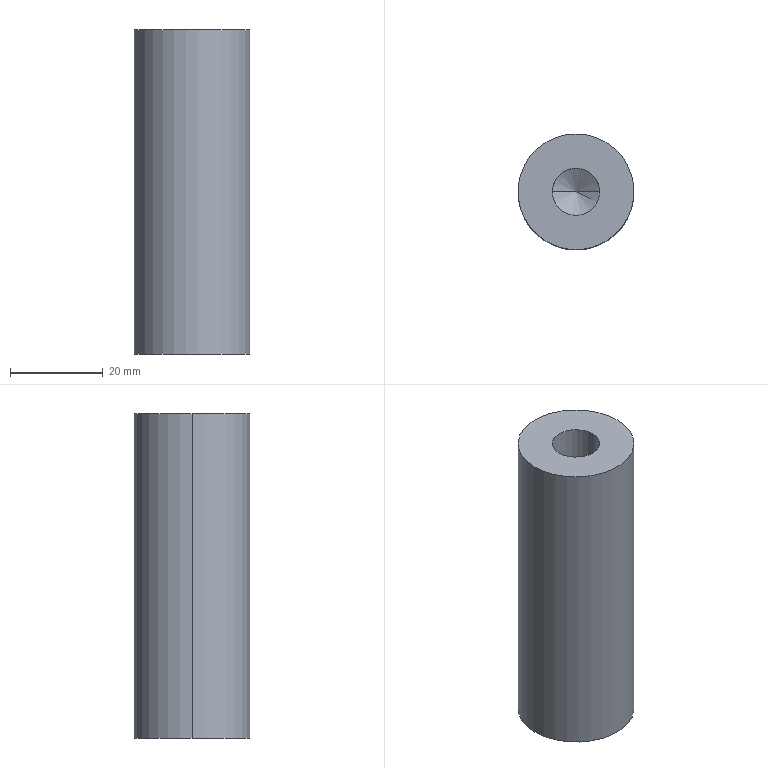Part | SolidWorks | features HoleWzd 2, Extrusion 1 | 1 solid | 12 faces | box 25 x 25 x 70 mm | volume 29291 mm3 | cylinder 6 | cone 4 | plane 2 | commonest cylinder face diameters 10.2 x4 25 x2
STEP:
#1=CARTESIAN_POINT('',(5.1,0.,30.));
#2=VERTEX_POINT('',#1);
#3=CARTESIAN_POINT('',(-5.1,0.,30.));
#4=VERTEX_POINT('',#3);
#5=CARTESIAN_POINT('',(0.,0.,30.));
#6=DIRECTION('',(0.,0.,-1.));
#7=DIRECTION('',(-1.,0.,0.));
#8=AXIS2_PLACEMENT_3D('',#5,#6,#7);
#9=CIRCLE('',#8,5.1);
#10=EDGE_CURVE('',#2,#4,#9,.T.);
#11=ORIENTED_EDGE('',*,*,#10,.F.);
#12=CARTESIAN_POINT('',(5.1,0.,0.));
#13=VERTEX_POINT('',#12);
#14=CARTESIAN_POINT('',(5.1,0.,0.));
#15=DIRECTION('',(0.,0.,-1.));
#16=VECTOR('',#15,1000.);
#17=LINE('',#14,#16);
#18=EDGE_CURVE('',#2,#13,#17,.T.);
#19=ORIENTED_EDGE('',*,*,#18,.T.);
#20=CARTESIAN_POINT('',(-5.1,0.,0.));
#21=VERTEX_POINT('',#20);
#22=CARTESIAN_POINT('',(0.,0.,0.));
#23=DIRECTION('',(0.,0.,-1.));
#24=DIRECTION('',(-1.,0.,0.));
#25=AXIS2_PLACEMENT_3D('',#22,#23,#24);
#26=CIRCLE('',#25,5.1);
#27=EDGE_CURVE('',#13,#21,#26,.T.);
#28=ORIENTED_EDGE('',*,*,#27,.T.);
#29=CARTESIAN_POINT('',(-5.1,0.,0.));
#30=DIRECTION('',(0.,0.,-1.));
#31=VECTOR('',#30,1000.);
#32=LINE('',#29,#31);
#33=EDGE_CURVE('',#4,#21,#32,.T.);
#34=ORIENTED_EDGE('',*,*,#33,.F.);
#35=EDGE_LOOP('',(#11,#19,#28,#34));
#36=FACE_OUTER_BOUND('',#35,.T.);
#37=CARTESIAN_POINT('',(0.,0.,0.));
#38=DIRECTION('',(0.,0.,-1.));
#39=DIRECTION('',(-1.,0.,0.));
#40=AXIS2_PLACEMENT_3D('',#37,#38,#39);
#41=CYLINDRICAL_SURFACE('',#40,5.1);
#42=ADVANCED_FACE('',(#36),#41,.F.);
#43=CARTESIAN_POINT('',(0.,0.,33.064));
#44=VERTEX_POINT('',#43);
#45=CARTESIAN_POINT('',(-5.1,0.,30.));
#46=DIRECTION('',(-0.8572,0.,-0.515));
#47=VECTOR('',#46,1000.);
#48=LINE('',#45,#47);
#49=EDGE_CURVE('',#44,#4,#48,.T.);
#50=ORIENTED_EDGE('',*,*,#49,.F.);
#51=CARTESIAN_POINT('',(5.1,0.,30.));
#52=DIRECTION('',(0.8572,0.,-0.515));
#53=VECTOR('',#52,1000.);
#54=LINE('',#51,#53);
#55=EDGE_CURVE('',#44,#2,#54,.T.);
#56=ORIENTED_EDGE('',*,*,#55,.T.);
#57=ORIENTED_EDGE('',*,*,#10,.T.);
#58=EDGE_LOOP('',(#50,#56,#57));
#59=FACE_OUTER_BOUND('',#58,.T.);
#60=CARTESIAN_POINT('',(0.,0.,30.));
#61=DIRECTION('',(0.,0.,-1.));
#62=DIRECTION('',(-1.,0.,0.));
#63=AXIS2_PLACEMENT_3D('',#60,#61,#62);
#64=CONICAL_SURFACE('',#63,5.1,1.03);
#65=ADVANCED_FACE('',(#59),#64,.F.);
#66=CARTESIAN_POINT('',(-5.1,0.,40.));
#67=VERTEX_POINT('',#66);
#68=CARTESIAN_POINT('',(5.1,0.,40.));
#69=VERTEX_POINT('',#68);
#70=CARTESIAN_POINT('',(0.,0.,40.));
#71=DIRECTION('',(0.,0.,1.));
#72=DIRECTION('',(1.,0.,0.));
#73=AXIS2_PLACEMENT_3D('',#70,#71,#72);
#74=CIRCLE('',#73,5.1);
#75=EDGE_CURVE('',#67,#69,#74,.T.);
#76=ORIENTED_EDGE('',*,*,#75,.F.);
#77=CARTESIAN_POINT('',(-5.1,0.,70.));
#78=VERTEX_POINT('',#77);
#79=CARTESIAN_POINT('',(-5.1,0.,70.));
#80=DIRECTION('',(0.,0.,1.));
#81=VECTOR('',#80,1000.);
#82=LINE('',#79,#81);
#83=EDGE_CURVE('',#67,#78,#82,.T.);
#84=ORIENTED_EDGE('',*,*,#83,.T.);
#85=CARTESIAN_POINT('',(5.1,0.,70.));
#86=VERTEX_POINT('',#85);
#87=CARTESIAN_POINT('',(0.,0.,70.));
#88=DIRECTION('',(0.,0.,1.));
#89=DIRECTION('',(1.,0.,0.));
#90=AXIS2_PLACEMENT_3D('',#87,#88,#89);
#91=CIRCLE('',#90,5.1);
#92=EDGE_CURVE('',#78,#86,#91,.T.);
#93=ORIENTED_EDGE('',*,*,#92,.T.);
#94=CARTESIAN_POINT('',(5.1,0.,70.));
#95=DIRECTION('',(0.,0.,1.));
#96=VECTOR('',#95,1000.);
#97=LINE('',#94,#96);
#98=EDGE_CURVE('',#69,#86,#97,.T.);
#99=ORIENTED_EDGE('',*,*,#98,.F.);
#100=EDGE_LOOP('',(#76,#84,#93,#99));
#101=FACE_OUTER_BOUND('',#100,.T.);
#102=CARTESIAN_POINT('',(0.,0.,70.));
#103=DIRECTION('',(0.,0.,1.));
#104=DIRECTION('',(1.,0.,0.));
#105=AXIS2_PLACEMENT_3D('',#102,#103,#104);
#106=CYLINDRICAL_SURFACE('',#105,5.1);
#107=ADVANCED_FACE('',(#101),#106,.F.);
#108=CARTESIAN_POINT('',(0.,0.,36.936));
#109=VERTEX_POINT('',#108);
#110=CARTESIAN_POINT('',(5.1,0.,40.));
#111=DIRECTION('',(0.8572,0.,0.515));
#112=VECTOR('',#111,1000.);
#113=LINE('',#110,#112);
#114=EDGE_CURVE('',#109,#69,#113,.T.);
#115=ORIENTED_EDGE('',*,*,#114,.F.);
#116=CARTESIAN_POINT('',(-5.1,0.,40.));
#117=DIRECTION('',(-0.8572,0.,0.515));
#118=VECTOR('',#117,1000.);
#119=LINE('',#116,#118);
#120=EDGE_CURVE('',#109,#67,#119,.T.);
#121=ORIENTED_EDGE('',*,*,#120,.T.);
#122=ORIENTED_EDGE('',*,*,#75,.T.);
#123=EDGE_LOOP('',(#115,#121,#122));
#124=FACE_OUTER_BOUND('',#123,.T.);
#125=CARTESIAN_POINT('',(0.,0.,40.));
#126=DIRECTION('',(0.,0.,1.));
#127=DIRECTION('',(1.,0.,0.));
#128=AXIS2_PLACEMENT_3D('',#125,#126,#127);
#129=CONICAL_SURFACE('',#128,5.1,1.03);
#130=ADVANCED_FACE('',(#124),#129,.F.);
#131=CARTESIAN_POINT('',(12.5,0.,70.));
#132=VERTEX_POINT('',#131);
#133=CARTESIAN_POINT('',(-12.5,0.,70.));
#134=VERTEX_POINT('',#133);
#135=CARTESIAN_POINT('',(0.,0.,70.));
#136=DIRECTION('',(0.,0.,1.));
#137=DIRECTION('',(1.,0.,0.));
#138=AXIS2_PLACEMENT_3D('',#135,#136,#137);
#139=CIRCLE('',#138,12.5);
#140=EDGE_CURVE('',#132,#134,#139,.T.);
#141=ORIENTED_EDGE('',*,*,#140,.F.);
#142=CARTESIAN_POINT('',(12.5,0.,0.));
#143=VERTEX_POINT('',#142);
#144=CARTESIAN_POINT('',(12.5,0.,70.));
#145=DIRECTION('',(0.,0.,-1.));
#146=VECTOR('',#145,1000.);
#147=LINE('',#144,#146);
#148=EDGE_CURVE('',#132,#143,#147,.T.);
#149=ORIENTED_EDGE('',*,*,#148,.T.);
#150=CARTESIAN_POINT('',(-12.5,0.,0.));
#151=VERTEX_POINT('',#150);
#152=CARTESIAN_POINT('',(0.,0.,0.));
#153=DIRECTION('',(0.,0.,1.));
#154=DIRECTION('',(1.,0.,0.));
#155=AXIS2_PLACEMENT_3D('',#152,#153,#154);
#156=CIRCLE('',#155,12.5);
#157=EDGE_CURVE('',#143,#151,#156,.T.);
#158=ORIENTED_EDGE('',*,*,#157,.T.);
#159=CARTESIAN_POINT('',(-12.5,0.,70.));
#160=DIRECTION('',(0.,0.,-1.));
#161=VECTOR('',#160,1000.);
#162=LINE('',#159,#161);
#163=EDGE_CURVE('',#134,#151,#162,.T.);
#164=ORIENTED_EDGE('',*,*,#163,.F.);
#165=EDGE_LOOP('',(#141,#149,#158,#164));
#166=FACE_OUTER_BOUND('',#165,.T.);
#167=CARTESIAN_POINT('',(0.,0.,70.));
#168=DIRECTION('',(0.,0.,-1.));
#169=DIRECTION('',(-1.,0.,0.));
#170=AXIS2_PLACEMENT_3D('',#167,#168,#169);
#171=CYLINDRICAL_SURFACE('',#170,12.5);
#172=ADVANCED_FACE('',(#166),#171,.T.);
#173=ORIENTED_EDGE('',*,*,#148,.F.);
#174=CARTESIAN_POINT('',(0.,0.,70.));
#175=DIRECTION('',(0.,0.,1.));
#176=DIRECTION('',(1.,0.,0.));
#177=AXIS2_PLACEMENT_3D('',#174,#175,#176);
#178=CIRCLE('',#177,12.5);
#179=EDGE_CURVE('',#134,#132,#178,.T.);
#180=ORIENTED_EDGE('',*,*,#179,.F.);
#181=ORIENTED_EDGE('',*,*,#163,.T.);
#182=CARTESIAN_POINT('',(0.,0.,0.));
#183=DIRECTION('',(0.,0.,1.));
#184=DIRECTION('',(1.,0.,0.));
#185=AXIS2_PLACEMENT_3D('',#182,#183,#184);
#186=CIRCLE('',#185,12.5);
#187=EDGE_CURVE('',#151,#143,#186,.T.);
#188=ORIENTED_EDGE('',*,*,#187,.T.);
#189=EDGE_LOOP('',(#173,#180,#181,#188));
#190=FACE_OUTER_BOUND('',#189,.T.);
#191=CARTESIAN_POINT('',(0.,0.,70.));
#192=DIRECTION('',(0.,0.,-1.));
#193=DIRECTION('',(-1.,0.,0.));
#194=AXIS2_PLACEMENT_3D('',#191,#192,#193);
#195=CYLINDRICAL_SURFACE('',#194,12.5);
#196=ADVANCED_FACE('',(#190),#195,.T.);
#197=CARTESIAN_POINT('',(0.,0.,70.));
#198=DIRECTION('',(0.,0.,1.));
#199=DIRECTION('',(1.,0.,0.));
#200=AXIS2_PLACEMENT_3D('',#197,#198,#199);
#201=CIRCLE('',#200,5.1);
#202=EDGE_CURVE('',#86,#78,#201,.T.);
#203=ORIENTED_EDGE('',*,*,#202,.F.);
#204=ORIENTED_EDGE('',*,*,#92,.F.);
#205=EDGE_LOOP('',(#203,#204));
#206=FACE_BOUND('',#205,.T.);
#207=ORIENTED_EDGE('',*,*,#179,.T.);
#208=ORIENTED_EDGE('',*,*,#140,.T.);
#209=EDGE_LOOP('',(#207,#208));
#210=FACE_OUTER_BOUND('',#209,.T.);
#211=CARTESIAN_POINT('',(0.,0.,70.));
#212=DIRECTION('',(0.,0.,1.));
#213=DIRECTION('',(1.,0.,0.));
#214=AXIS2_PLACEMENT_3D('',#211,#212,#213);
#215=PLANE('',#214);
#216=ADVANCED_FACE('',(#206,#210),#215,.T.);
#217=CARTESIAN_POINT('',(0.,0.,0.));
#218=DIRECTION('',(0.,0.,-1.));
#219=DIRECTION('',(-1.,0.,0.));
#220=AXIS2_PLACEMENT_3D('',#217,#218,#219);
#221=CIRCLE('',#220,5.1);
#222=EDGE_CURVE('',#21,#13,#221,.T.);
#223=ORIENTED_EDGE('',*,*,#222,.F.);
#224=ORIENTED_EDGE('',*,*,#27,.F.);
#225=EDGE_LOOP('',(#223,#224));
#226=FACE_BOUND('',#225,.T.);
#227=ORIENTED_EDGE('',*,*,#187,.F.);
#228=ORIENTED_EDGE('',*,*,#157,.F.);
#229=EDGE_LOOP('',(#227,#228));
#230=FACE_OUTER_BOUND('',#229,.T.);
#231=CARTESIAN_POINT('',(0.,0.,0.));
#232=DIRECTION('',(0.,0.,1.));
#233=DIRECTION('',(1.,0.,0.));
#234=AXIS2_PLACEMENT_3D('',#231,#232,#233);
#235=PLANE('',#234);
#236=ADVANCED_FACE('',(#226,#230),#235,.F.);
#237=ORIENTED_EDGE('',*,*,#120,.F.);
#238=ORIENTED_EDGE('',*,*,#114,.T.);
#239=CARTESIAN_POINT('',(0.,0.,40.));
#240=DIRECTION('',(0.,0.,1.));
#241=DIRECTION('',(1.,0.,0.));
#242=AXIS2_PLACEMENT_3D('',#239,#240,#241);
#243=CIRCLE('',#242,5.1);
#244=EDGE_CURVE('',#69,#67,#243,.T.);
#245=ORIENTED_EDGE('',*,*,#244,.T.);
#246=EDGE_LOOP('',(#237,#238,#245));
#247=FACE_OUTER_BOUND('',#246,.T.);
#248=CARTESIAN_POINT('',(0.,0.,40.));
#249=DIRECTION('',(0.,0.,1.));
#250=DIRECTION('',(1.,0.,0.));
#251=AXIS2_PLACEMENT_3D('',#248,#249,#250);
#252=CONICAL_SURFACE('',#251,5.1,1.03);
#253=ADVANCED_FACE('',(#247),#252,.F.);
#254=ORIENTED_EDGE('',*,*,#83,.F.);
#255=ORIENTED_EDGE('',*,*,#244,.F.);
#256=ORIENTED_EDGE('',*,*,#98,.T.);
#257=ORIENTED_EDGE('',*,*,#202,.T.);
#258=EDGE_LOOP('',(#254,#255,#256,#257));
#259=FACE_OUTER_BOUND('',#258,.T.);
#260=CARTESIAN_POINT('',(0.,0.,70.));
#261=DIRECTION('',(0.,0.,1.));
#262=DIRECTION('',(1.,0.,0.));
#263=AXIS2_PLACEMENT_3D('',#260,#261,#262);
#264=CYLINDRICAL_SURFACE('',#263,5.1);
#265=ADVANCED_FACE('',(#259),#264,.F.);
#266=ORIENTED_EDGE('',*,*,#55,.F.);
#267=ORIENTED_EDGE('',*,*,#49,.T.);
#268=CARTESIAN_POINT('',(0.,0.,30.));
#269=DIRECTION('',(0.,0.,-1.));
#270=DIRECTION('',(-1.,0.,0.));
#271=AXIS2_PLACEMENT_3D('',#268,#269,#270);
#272=CIRCLE('',#271,5.1);
#273=EDGE_CURVE('',#4,#2,#272,.T.);
#274=ORIENTED_EDGE('',*,*,#273,.T.);
#275=EDGE_LOOP('',(#266,#267,#274));
#276=FACE_OUTER_BOUND('',#275,.T.);
#277=CARTESIAN_POINT('',(0.,0.,30.));
#278=DIRECTION('',(0.,0.,-1.));
#279=DIRECTION('',(-1.,0.,0.));
#280=AXIS2_PLACEMENT_3D('',#277,#278,#279);
#281=CONICAL_SURFACE('',#280,5.1,1.03);
#282=ADVANCED_FACE('',(#276),#281,.F.);
#283=ORIENTED_EDGE('',*,*,#18,.F.);
#284=ORIENTED_EDGE('',*,*,#273,.F.);
#285=ORIENTED_EDGE('',*,*,#33,.T.);
#286=ORIENTED_EDGE('',*,*,#222,.T.);
#287=EDGE_LOOP('',(#283,#284,#285,#286));
#288=FACE_OUTER_BOUND('',#287,.T.);
#289=CARTESIAN_POINT('',(0.,0.,0.));
#290=DIRECTION('',(0.,0.,-1.));
#291=DIRECTION('',(-1.,0.,0.));
#292=AXIS2_PLACEMENT_3D('',#289,#290,#291);
#293=CYLINDRICAL_SURFACE('',#292,5.1);
#294=ADVANCED_FACE('',(#288),#293,.F.);
#295=CLOSED_SHELL('',(#42,#65,#107,#130,#172,#196,#216,#236,#253,#265,#282,#294));
#296=MANIFOLD_SOLID_BREP('',#295);
#297=CARTESIAN_POINT('',(0.,0.,0.));
#298=DIRECTION('',(0.,0.,1.));
#299=DIRECTION('',(1.,0.,0.));
#300=AXIS2_PLACEMENT_3D('',#297,#298,#299);
#301=(LENGTH_UNIT()NAMED_UNIT(*)SI_UNIT(.MILLI.,.METRE.));
#302=UNCERTAINTY_MEASURE_WITH_UNIT(LENGTH_MEASURE(0.00001),#301,'','');
#303=(NAMED_UNIT(*)PLANE_ANGLE_UNIT()SI_UNIT($,.RADIAN.));
#304=(NAMED_UNIT(*)SI_UNIT($,.STERADIAN.)SOLID_ANGLE_UNIT());
#305=(GEOMETRIC_REPRESENTATION_CONTEXT(3)GLOBAL_UNCERTAINTY_ASSIGNED_CONTEXT((#302))GLOBAL_UNIT_ASSIGNED_CONTEXT((#301,#303,#304))REPRESENTATION_CONTEXT('',''));
#306=ADVANCED_BREP_SHAPE_REPRESENTATION('',(#296,#300),#305);